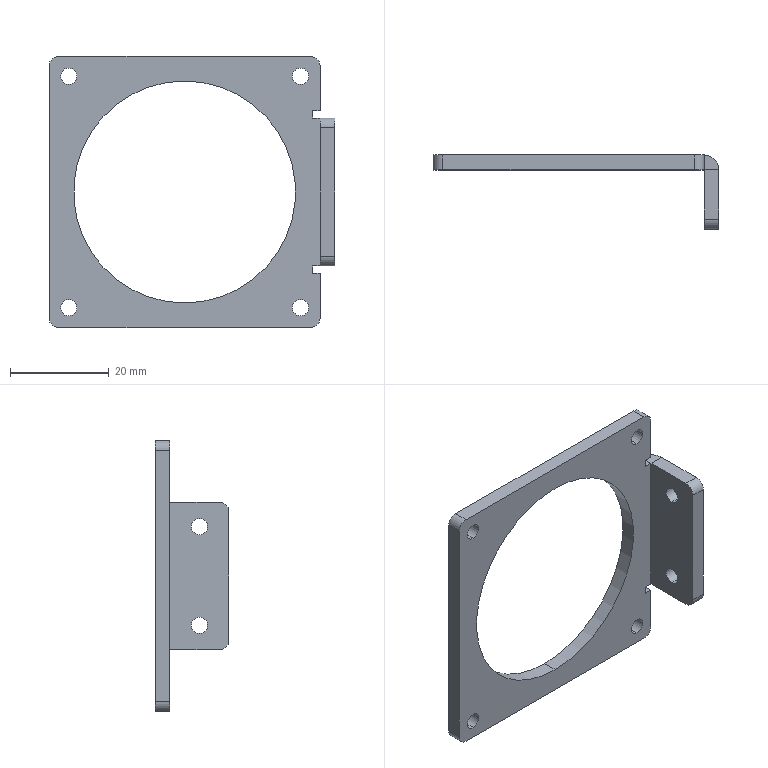Part | STEP file | motor mounting sheet metal 2 | 1 solid | 42 faces | box 58 x 15 x 55 mm | volume 5412 mm3 | cylinder 22 | plane 20 | commonest cylinder face diameters 3.3 x12 4 x6 45 x2 0.02 x1 6.02 x1